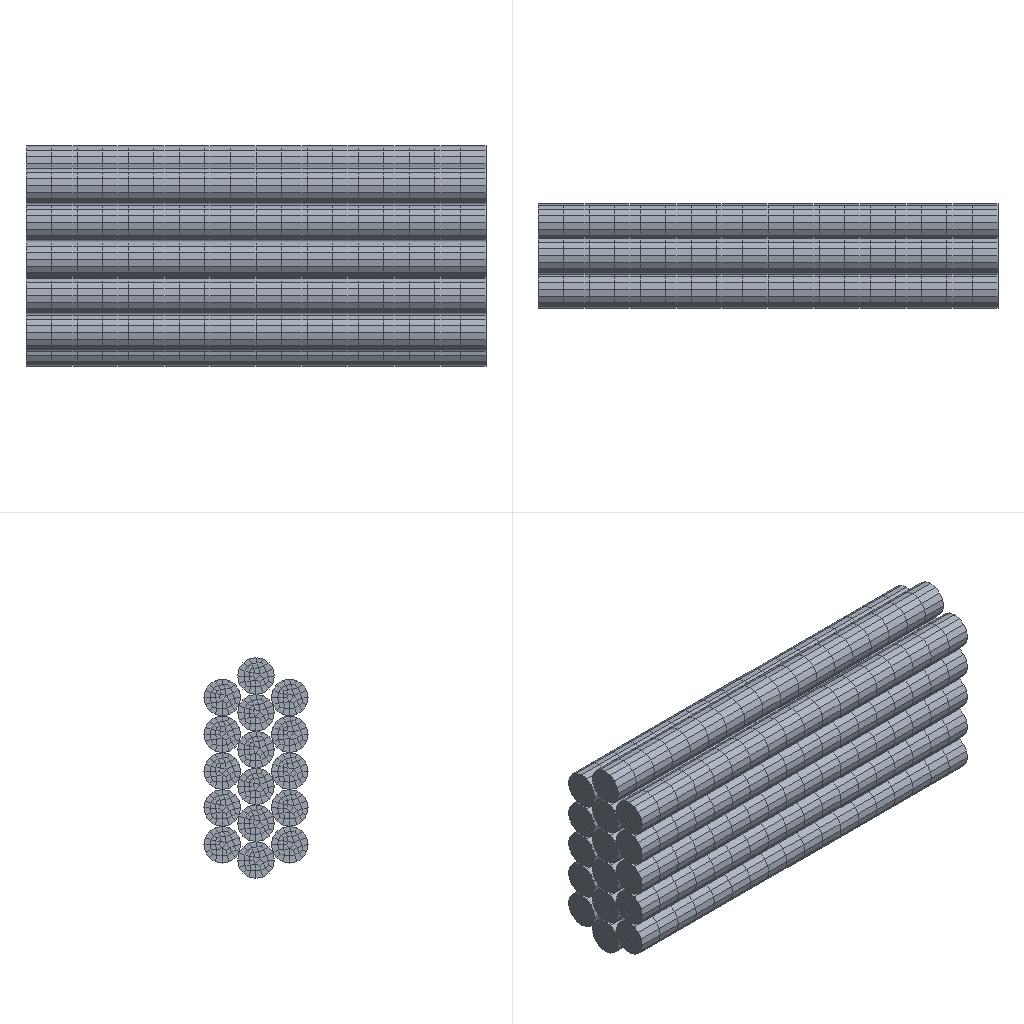Simulation study | abaqus
Set-up summary:
category,name,step,type,value,unit,region
solver,abaqus
solver,version,,,Abaqus/Explicit 2020
units,not stated in the deck,,not stated
analysis,deck,,transient,transient
load_step,Step-1,Step-1,transient
load_step,requested,,,1
mesh,nodes,,,15325
mesh,elements,,,12032
element_type,R3D3,,rigid,30
element_type,R3D4,,rigid,1922
element_type,C3D8RT,,solid,10080
load,load commands in deck,,count,3
bc,support commands in deck,,count,10
material,MATERIAL-1,,in results
check,setup vs results,,match,"per instance, exact: element labels, types and connectivity; labels of the nodes the elements use; coordinates not compared"
Abaqus input file, long lists of numbers shortened:
*Heading
** Job name: Job-1 Model name: Model-1
** Generated by: Abaqus/CAE 2020
*Preprint, echo=NO, model=NO, history=NO, contact=NO
**
** PARTS
**
*Part, name=dang
*Node
      1,           0.,           0.,           0.
      2,           0.,         -2.5,           0.
** (130 more lines like these left out)
*Element, type=R3D4
1,  1,  9, 16,  4
2,  9, 10, 15, 16
** (128 more lines like these left out)
*Node
    133,          2.5,           0.,          0.5
*Nset, nset=dang-RefPt_, internal
133,
*Elset, elset=dang, generate
   1,  130,    1
*End Part
**
*Part, name=under
*Node
      1,  0.6,           0.,           0.
      2,           0.,           0.,           0.
** (937 more lines like these left out)
*Element, type=R3D4
 1,   1,  33, 285,  58
 2,  33,  34, 286, 285
** (926 more lines like these left out)
*Element, type=R3D3
683, 782, 758, 753
684, 784, 755, 757
** (16 more lines like these left out)
*Node
    940,   2.7,          -1.,           0.
*Nset, nset=under-RefPt_, internal
940,
*Elset, elset=under, generate
   1,  946,    1
*End Part
**
*Part, name=up
*Node
      1,           0.,          -1.,           0.
      2,    5.4,          -1.,           0.
** (740 more lines like these left out)
*Element, type=R3D4
  1,   1,  33, 255,  88
  2,  33,  34, 256, 255
** (732 more lines like these left out)
*Element, type=R3D3
551, 607, 646, 629
552, 632, 612, 622
** (10 more lines like these left out)
*Node
    743,   2.7,          -1.,   2.8
*Nset, nset=up-RefPt_, internal
743,
*Elset, elset=up, generate
   1,  746,    1
*End Part
**
*Part, name=work
*Node
      1,           0., 0.09184, -0.2217
      2,           0.,  0.2217, -0.09184
** (834 more lines like these left out)
*Element, type=C3D8RT
  1,  18,   2,  13,  27,  62,  46,  57,  71
  2,   2,  18,  30,   3,  46,  62,  74,  47
** (628 more lines like these left out)
*Nset, nset=Set-4, generate
   1,  836,    1
*Elset, elset=Set-4, generate
   1,  630,    1
** Section: Section-1
*Solid Section, elset=Set-4, material=Material-1
,
*End Part
**
**
** ASSEMBLY
**
*Assembly, name=Assembly
**
*Instance, name=work-1, part=work
         5.9,         0.55,         0.45
*End Instance
**
*Instance, name=work-1-lin-1-2, part=work
         5.9, 0.55,         0.93
*End Instance
**
*Instance, name=work-1-lin-1-3, part=work
         5.9, 0.55,         1.41
*End Instance
**
*Instance, name=work-1-lin-1-4, part=work
         5.9, 0.55,         1.89
*End Instance
**
*Instance, name=work-1-lin-1-5, part=work
         5.9, 0.55,         2.37
*End Instance
**
*Instance, name=work-2, part=work
         5.9,         0.99,         0.25
*End Instance
**
*Instance, name=work-2-lin-1-2, part=work
         5.9,         0.99,         0.73
*End Instance
**
*Instance, name=work-2-lin-1-3, part=work
         5.9,         0.99,         1.21
*End Instance
**
*Instance, name=work-2-lin-1-4, part=work
         5.9,         0.99,         1.69
*End Instance
**
*Instance, name=work-2-lin-1-5, part=work
         5.9,         0.99,         2.17
*End Instance
**
*Instance, name=work-2-lin-1-6, part=work
         5.9,         0.99,         2.65
*End Instance
**
*Instance, name=work-3, part=work
         5.9,         1.43,         0.45
*End Instance
**
*Instance, name=work-3-lin-1-2, part=work
         5.9,         1.43,         0.93
*End Instance
**
*Instance, name=work-3-lin-1-3, part=work
         5.9,         1.43,         1.41
*End Instance
**
*Instance, name=work-3-lin-1-4, part=work
         5.9,         1.43,         1.89
*End Instance
**
*Instance, name=work-3-lin-1-5, part=work
         5.9,         1.43,         2.37
*End Instance
**
*Instance, name=under-2, part=under
*End Instance
**
*Instance, name=dang-3, part=dang
         0.3,          2.8,         -0.5
*End Instance
**
*Instance, name=dang-4, part=dang
         0.3,          2.8,          2.9
*End Instance
**
*Instance, name=up-2, part=up
          0.,          1.7,         2.85
          0.,          1.7,         2.85,           1.,          1.7,         2.85,         180.
*End Instance
**
*Nset, nset=Set-1, instance=under-2
   5,   6,   7,   8,  62,  63,  64,  65,  66,  67,  68,  69,  70,  71,  75,  76
  77,  78,  79,  80,  81,  82,  83,  84,  85,  86,  87,  88,  89,  90,  91,  92
** (14 more lines like these left out)
*Nset, nset=Set-1, instance=dang-3
  2,  3,  5,  6, 17, 18, 19, 20, 21, 22, 23, 24, 25, 26, 27, 28
 29, 30, 31, 32, 33, 34
*Nset, nset=Set-1, instance=dang-4
  2,  3,  5,  6, 17, 18, 19, 20, 21, 22, 23, 24, 25, 26, 27, 28
 29, 30, 31, 32, 33, 34
*Elset, elset=Set-1, instance=under-2, generate
  89,  308,    1
*Elset, elset=Set-1, instance=dang-3, generate
  6,  15,   1
*Elset, elset=Set-1, instance=dang-4, generate
  6,  15,   1
*Nset, nset=Set-2, instance=work-1, generate
   1,  836,    1
*Nset, nset=Set-2, instance=work-1-lin-1-2, generate
   1,  836,    1
*Nset, nset=Set-2, instance=work-1-lin-1-3, generate
   1,  836,    1
*Nset, nset=Set-2, instance=work-2-lin-1-2, generate
   1,  836,    1
*Nset, nset=Set-2, instance=work-2-lin-1-6, generate
   1,  836,    1
*Nset, nset=Set-2, instance=work-3-lin-1-4, generate
   1,  836,    1
*Nset, nset=Set-2, instance=work-1-lin-1-5, generate
   1,  836,    1
*Nset, nset=Set-2, instance=work-3-lin-1-2, generate
   1,  836,    1
*Nset, nset=Set-2, instance=work-2-lin-1-4, generate
   1,  836,    1
*Nset, nset=Set-2, instance=work-1-lin-1-4, generate
   1,  836,    1
*Nset, nset=Set-2, instance=work-2-lin-1-3, generate
   1,  836,    1
*Nset, nset=Set-2, instance=work-3, generate
   1,  836,    1
*Nset, nset=Set-2, instance=work-3-lin-1-5, generate
   1,  836,    1
*Nset, nset=Set-2, instance=work-2, generate
   1,  836,    1
*Nset, nset=Set-2, instance=work-3-lin-1-3, generate
   1,  836,    1
*Nset, nset=Set-2, instance=work-2-lin-1-5, generate
   1,  836,    1
*Elset, elset=Set-2, instance=work-1, generate
   1,  630,    1
*Elset, elset=Set-2, instance=work-1-lin-1-2, generate
   1,  630,    1
*Elset, elset=Set-2, instance=work-1-lin-1-3, generate
   1,  630,    1
*Elset, elset=Set-2, instance=work-2-lin-1-2, generate
   1,  630,    1
*Elset, elset=Set-2, instance=work-2-lin-1-6, generate
   1,  630,    1
*Elset, elset=Set-2, instance=work-3-lin-1-4, generate
   1,  630,    1
*Elset, elset=Set-2, instance=work-1-lin-1-5, generate
   1,  630,    1
*Elset, elset=Set-2, instance=work-3-lin-1-2, generate
   1,  630,    1
*Elset, elset=Set-2, instance=work-2-lin-1-4, generate
   1,  630,    1
*Elset, elset=Set-2, instance=work-1-lin-1-4, generate
   1,  630,    1
*Elset, elset=Set-2, instance=work-2-lin-1-3, generate
   1,  630,    1
*Elset, elset=Set-2, instance=work-3, generate
   1,  630,    1
*Elset, elset=Set-2, instance=work-3-lin-1-5, generate
   1,  630,    1
*Elset, elset=Set-2, instance=work-2, generate
   1,  630,    1
*Elset, elset=Set-2, instance=work-3-lin-1-3, generate
   1,  630,    1
*Elset, elset=Set-2, instance=work-2-lin-1-5, generate
   1,  630,    1
*Nset, nset=Set-3, instance=work-1, generate
  1,  44,   1
*Nset, nset=Set-3, instance=work-1-lin-1-2, generate
  1,  44,   1
*Nset, nset=Set-3, instance=work-1-lin-1-3, generate
  1,  44,   1
*Nset, nset=Set-3, instance=work-2-lin-1-2, generate
  1,  44,   1
*Nset, nset=Set-3, instance=work-2-lin-1-6, generate
  1,  44,   1
*Nset, nset=Set-3, instance=work-3-lin-1-4, generate
  1,  44,   1
*Nset, nset=Set-3, instance=work-1-lin-1-5, generate
  1,  44,   1
*Nset, nset=Set-3, instance=work-3-lin-1-2, generate
  1,  44,   1
*Nset, nset=Set-3, instance=work-2-lin-1-4, generate
  1,  44,   1
*Nset, nset=Set-3, instance=work-1-lin-1-4, generate
  1,  44,   1
*Nset, nset=Set-3, instance=work-2-lin-1-3, generate
  1,  44,   1
*Nset, nset=Set-3, instance=work-3, generate
  1,  44,   1
*Nset, nset=Set-3, instance=work-3-lin-1-5, generate
  1,  44,   1
*Nset, nset=Set-3, instance=work-2, generate
  1,  44,   1
*Nset, nset=Set-3, instance=work-3-lin-1-3, generate
  1,  44,   1
*Nset, nset=Set-3, instance=work-2-lin-1-5, generate
  1,  44,   1
*Elset, elset=Set-3, instance=work-1, generate
  1,  35,   1
*Elset, elset=Set-3, instance=work-1-lin-1-2, generate
  1,  35,   1
*Elset, elset=Set-3, instance=work-1-lin-1-3, generate
  1,  35,   1
*Elset, elset=Set-3, instance=work-2-lin-1-2, generate
  1,  35,   1
*Elset, elset=Set-3, instance=work-2-lin-1-6, generate
  1,  35,   1
*Elset, elset=Set-3, instance=work-3-lin-1-4, generate
  1,  35,   1
*Elset, elset=Set-3, instance=work-1-lin-1-5, generate
  1,  35,   1
*Elset, elset=Set-3, instance=work-3-lin-1-2, generate
  1,  35,   1
*Elset, elset=Set-3, instance=work-2-lin-1-4, generate
  1,  35,   1
*Elset, elset=Set-3, instance=work-1-lin-1-4, generate
  1,  35,   1
*Elset, elset=Set-3, instance=work-2-lin-1-3, generate
  1,  35,   1
*Elset, elset=Set-3, instance=work-3, generate
  1,  35,   1
*Elset, elset=Set-3, instance=work-3-lin-1-5, generate
  1,  35,   1
*Elset, elset=Set-3, instance=work-2, generate
  1,  35,   1
*Elset, elset=Set-3, instance=work-3-lin-1-3, generate
  1,  35,   1
*Elset, elset=Set-3, instance=work-2-lin-1-5, generate
  1,  35,   1
*Nset, nset=Set-4, instance=up-2
 743,
*Nset, nset=Set-5, instance=dang-3
 133,
*Nset, nset=Set-6, instance=dang-4
 133,
*Nset, nset=Set-7, instance=under-2
 940,
*Nset, nset=Set-8, instance=up-2
   1,   2,   3,   4,  33,  34,  35,  36,  37,  38,  39,  40,  41,  42,  43,  44
  45,  46,  47,  48,  49,  50,  51,  52,  53,  54,  55,  56,  57,  58,  59,  60
** (13 more lines like these left out)
*Elset, elset=Set-8, instance=up-2, generate
   1,  200,    1
*Nset, nset=Set-9, instance=up-2
 743,
*Nset, nset=Set-10, instance=up-2
 743,
*Nset, nset=Set-11, instance=up-2
 743,
*Elset, elset=_Surf-1_SPOS, internal, instance=up-2, generate
   1,  200,    1
*Surface, type=ELEMENT, name=Surf-1
_Surf-1_SPOS, SPOS
*Rigid Body, ref node=under-2.under-RefPt_, elset=under-2.under
*Rigid Body, ref node=dang-3.dang-RefPt_, elset=dang-3.dang
*Rigid Body, ref node=dang-4.dang-RefPt_, elset=dang-4.dang
*Rigid Body, ref node=up-2.up-RefPt_, elset=up-2.up
*End Assembly
*Amplitude, name=Amp-1, definition=PERIODIC
1,          12800.,              0.,              0.
           599.,              0.
**
** MATERIALS
**
*Material, name=Material-1
*Conductivity
110.,
*Density
 8.53e-09,
*Elastic
110000., 0.3
*Expansion
 2.02e-05,
*Plastic
125.,   0.
205., 0.02
255., 0.03
270., 0.04
280., 0.05
300., 0.06
310., 0.07
325., 0.08
340., 0.09
350.,  0.1
413.,  0.2
451.,  0.3
477.,  0.4
498.,  0.5
515.,  0.6
529.,  0.7
541.,  0.8
552.,  0.9
562.,   1.
*Specific Heat
 3.8e+08,
**
** INTERACTION PROPERTIES
**
*Surface Interaction, name=IntProp-1
*Friction
 0.3,
*Surface Behavior, pressure-overclosure=HARD
*Gap Heat Generation
1., 0.5
**
** BOUNDARY CONDITIONS
**
** Name: BC-2 Type: 对称/反对称/完全固定
*Boundary
Set-3, ENCASTRE
** Name: BC-4 Type: 对称/反对称/完全固定
*Boundary
Set-5, ENCASTRE
** Name: BC-5 Type: 对称/反对称/完全固定
*Boundary
Set-6, ENCASTRE
** Name: BC-6 Type: 对称/反对称/完全固定
*Boundary
Set-7, ENCASTRE
**
** PREDEFINED FIELDS
**
** Name: Predefined Field-1   Type: Temperature
*Initial Conditions, type=TEMPERATURE
Set-2, 25.
** ----------------------------------------------------------------
**
** STEP: Step-1
**
*Step, name=Step-1, nlgeom=YES
*Dynamic, Explicit
, 0.5
*Bulk Viscosity
0.06, 1.2
** Mass Scaling: Semi-Automatic
**               Whole Model
*Fixed Mass Scaling, dt=1e-05, type=below min
**
** BOUNDARY CONDITIONS
**
** Name: BC-3 Type: 速度/角速度
*Boundary, amplitude=Amp-1, type=VELOCITY
Set-4, 1, 1, 1.
Set-4, 3, 3
Set-4, 4, 4
Set-4, 5, 5
Set-4, 6, 6
** Name: BC-7 Type: 速度/角速度
*Boundary, type=VELOCITY
Set-11, 2, 2, -0.4
**
** LOADS
**
** Name: Load-1   Type: Concentrated force
*Cload
Set-10, 2, -60.
**
** INTERACTIONS
**
** Interaction: Int-1
*Contact, op=NEW
*Contact Inclusions, ALL EXTERIOR
*Contact Property Assignment
 ,  , IntProp-1
**
** OUTPUT REQUESTS
**
*Restart, write, number interval=1, time marks=NO
**
** FIELD OUTPUT: F-Output-1
**
*Output, field, number interval=200
*Node Output
A, RF, U, V
*Element Output, directions=YES
E, LE, MISES, PE, PEEQ, PEEQVAVG, PEVAVG, S, STATUS, SVAVG, TEMP
*Contact Output
CSTRESS,
**
** HISTORY OUTPUT: H-Output-1
**
*Output, history, variable=PRESELECT
*End Step
Results summary:
result,step,Step-1,completed,increments=41705 time=0.5/0.5
result,analysis,,,transient
result,last_loadstep,,,1
result,primary field,,,U
result,reaction total,,FX,-64.293,model units
result,reaction total,,FY,231.865,model units
result,reaction total,,FZ,35.201,model units